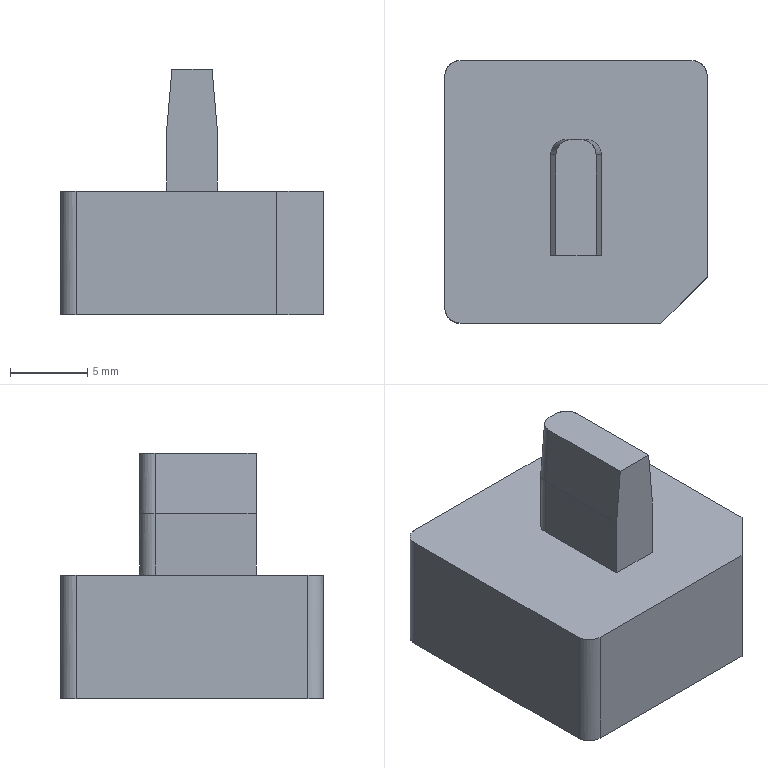NC program | PowerMill | posted with a generic post | part box 17 x 17 x 15.883 mm
Lines 2786 to 3249 of 22972:
N2883 M6
N2884 S8500 M03
N2885 G00 G90 X0.0 Y0.0
N2886 G43 Z11.804 H3
N2887
N2888 G05 P10000 R8
N2889 X11.8334 Y-1.5183
N2890 Z0.8029
N2891 G01 Z-0.3971 F360.0
N2892 X6.5584 F600.0
N2893 X2.4866 Y-1.3941
N2894 X2.4829 Y-1.1993
N2895 X2.4601 Y-1.0057
N2896 X2.0806 Y1.2544
N2897 G03 X-1.4275 Y1.6248 I-1.8056 J-0.3032
N2898 G01 X-2.3187 Y-0.6277
N2899 G03 X-0.431 Y-3.3368 I1.842 J-0.7288
N2900 G01 X0.5523 Y-3.3141
N2901 G03 X2.4866 Y-1.3941 I-0.0457 J1.9804
N2902 G01 X6.5584 Y-1.5183
N2903 G00 Z11.804
N2904 G05 P0
N2905 (---------------)
N2906 ( END TOOLPATH : 粗公基准台01-平坦面偏置-D10 )
N2907 (---------------)
N2908 ( START TOOLPATH : 粗公基准台01-基准面偏置-D10 )
N2909 (---------------)
N2910 G00 X0.0 Y0.0 Z9.8056
N2911 G05 P10000 R8
N2912 X-15.001 Y16.2619
N2913 Z-6.88
N2914 G01 Z-8.08 F360.0
N2915 X-11.5862 Y12.2414 F600.0
N2916 X-6.8885 Y2.4254
N2917 X-6.8737 Y2.7888
N2918 X-6.842 Y3.1512
N2919 G02 X-6.6309 Y4.1515 I5.9397 J-0.7309
N2920 G02 X-6.3033 Y5.0267 I5.8927 J-1.7068
N2921 G01 X-6.1678 Y5.3005
N2922 X-5.9818 Y5.6235
N2923 X-5.7814 Y5.9378
N2924 X-5.6173 Y6.1643
N2925 G02 X-4.8971 Y6.9601 I5.4256 J-4.1864
N2926 G01 X-4.5867 Y7.2255
N2927 X-4.2643 Y7.4761
N2928 X-4.0176 Y7.6439
N2929 G02 X-3.1431 Y8.1122 I3.7067 J-5.8707
N2930 G01 X-2.8431 Y8.234
N2931 G02 X-2.018 Y8.4819 I2.8305 J-7.9259
N2932 G02 X-0.6352 Y8.6371 I1.4581 J-6.7525
N2933 G01 X0.6352
N2934 X1.0035 Y8.6242
N2935 G02 X3.7983 Y7.7732 I-0.3537 J-6.1771
N2936 G02 X4.6028 Y7.212 I-2.6823 J-4.7021
N2937 G02 X6.52 Y4.4929 I-3.9063 J-4.7898
N2938 G02 X6.8891 Y2.3871 I-5.9216 J-2.1229
N2939 G01 Y-4.15
N2940 X6.8744 Y-4.5423
N2941 G02 X6.7574 Y-5.3182 I-6.1404 J0.5287
N2942 G01 X6.6558 Y-5.6975
N2943 X6.5262 Y-6.068
N2944 X6.3691 Y-6.4279
N2945 X6.1857 Y-6.775
N2946 X5.9768 Y-7.1074
N2947 X5.7585 Y-7.4033
N2948 X5.5917 Y-7.6028
N2949 X5.4149 Y-7.7936
N2950 X5.21 Y-7.9985
N2951 X4.9124 Y-8.2546
N2952 X4.5965 Y-8.4877
N2953 G02 X3.917 Y-8.8801 I-3.4465 J5.1847
N2954 G02 X2.8073 Y-9.2684 I-2.3879 J5.0442
N2955 G02 X2.0314 Y-9.3853 I-1.3291 J6.1858
N2956 G01 X1.6391 Y-9.4
N2957 X-1.6391
N2958 G02 X-2.4215 Y-9.3414 I0.0713 J6.2014
N2959 G01 X-2.8073 Y-9.2684
N2960 G02 X-3.5571 Y-9.0371 I1.4757 J6.115
N2961 G02 X-4.2641 Y-8.6966 I2.3236 J5.7292
N2962 G01 X-4.5965 Y-8.4878
N2963 G02 X-5.21 Y-7.9985 I3.6159 J5.1634
N2964 G02 X-5.7437 Y-7.4233 I4.3435 J4.5653
N2965 G01 X-5.9768 Y-7.1074
N2966 X-6.1857 Y-6.775
N2967 X-6.3691 Y-6.4279
N2968 X-6.5261 Y-6.068
N2969 X-6.6558 Y-5.6975
N2970 G02 X-6.8304 Y-4.9325 I6.0732 J1.7886
N2971 G01 X-6.8744 Y-4.5423
N2972 X-6.8891 Y-4.15
N2973 X-6.8885 Y2.4254
N2974 G00 Z9.8056
N2975 G05 P0
N2976 (---------------)
N2977 ( END TOOLPATH : 粗公基准台01-基准面偏置-D10 )
N2978 (---------------)
N2979 ( START TOOLPATH : 粗公基准台01-基准台侧光-D10 )
N2980 (---------------)
N2981 G00 X0.0 Y0.0 Z9.8056
N2982 G05 P10000 R8
N2983 X13.4803 Y-14.7747
N2984 Z-14.78
N2985 G01 Z-15.98 F360.0
N2986 G03 X9.9447 Y-11.2392 I-1.7678 J1.7678 F600.0
N2987 G01 X9.0587 Y-12.1252
N2988 X9.0582 Y-12.1257
N2989 X9.0577 Y-12.1262
N2990 X8.9953 Y-12.1864
N2991 X8.9933 Y-12.1883
N2992 X8.9913 Y-12.19
N2993 X8.5443 Y-12.5666
N2994 X8.5408 Y-12.5694
N2995 X8.5371 Y-12.572
N2996 X8.0901 Y-12.87
N2997 X8.0872 Y-12.8719
N2998 X8.0842 Y-12.8736
N2999 X7.7935 Y-13.0328
N3000 X7.7918 Y-13.0337
N3001 X7.79 Y-13.0346
N3002 X7.6336 Y-13.1102
N3003 X7.6312 Y-13.1114
N3004 X7.6288 Y-13.1124
N3005 X7.1818 Y-13.2935
N3006 X7.1783 Y-13.2948
N3007 X7.1746 Y-13.296
N3008 X6.7277 Y-13.4293
N3009 X6.7248 Y-13.4301
N3010 X6.722 Y-13.4308
N3011 X6.4639 Y-13.4877
N3012 X6.4621 Y-13.4881
N3013 X6.4603 Y-13.4884
N3014 X6.2714 Y-13.5211
N3015 X6.2689 Y-13.5215
N3016 X6.2664 Y-13.5218
N3017 X5.8194 Y-13.5699
N3018 X5.816 Y-13.5702
N3019 X5.8125 Y-13.5704
N3020 X5.3656 Y-13.58
N3021 X5.3647
N3022 X5.3638
N3023 X-7.5988 Y-13.5791
N3024 X-7.6011 Y-13.579
N3025 X-7.6033 Y-13.5789
N3026 X-8.0503 Y-13.5532
N3027 X-8.053 Y-13.553
N3028 X-8.0557 Y-13.5527
N3029 X-8.5027 Y-13.4965
N3030 X-8.5059 Y-13.496
N3031 X-8.5091 Y-13.4954
N3032 X-8.9561 Y-13.4017
N3033 X-8.9589 Y-13.4011
N3034 X-8.9617 Y-13.4003
N3035 X-9.4087 Y-13.2723
N3036 X-9.4118 Y-13.2713
N3037 X-9.4148 Y-13.2703
N3038 X-9.8618 Y-13.1025
N3039 X-9.8649 Y-13.1013
N3040 X-9.8679 Y-13.0999
N3041 X-10.3149 Y-12.8887
N3042 X-10.3178 Y-12.8872
N3043 X-10.3208 Y-12.8856
N3044 X-10.7677 Y-12.6268
N3045 X-10.7708 Y-12.6249
N3046 X-10.7738 Y-12.6229
N3047 X-11.2208 Y-12.3073
N3048 X-11.2238 Y-12.3051
N3049 X-11.2266 Y-12.3027
N3050 X-11.6736 Y-11.9205
N3051 X-11.676 Y-11.9184
N3052 X-11.6782 Y-11.9163
N3053 X-11.9163 Y-11.6782
N3054 X-11.9184 Y-11.676
N3055 X-11.9205 Y-11.6736
N3056 X-12.3027 Y-11.2266
N3057 X-12.3049 Y-11.224
N3058 X-12.307 Y-11.2213
N3059 X-12.5806 Y-10.8396
N3060 X-12.5827 Y-10.8365
N3061 X-12.5846 Y-10.8334
N3062 X-12.8853 Y-10.3212
N3063 X-12.8871 Y-10.318
N3064 X-12.8887 Y-10.3149
N3065 X-13.0999 Y-9.8679
N3066 X-13.1013 Y-9.8649
N3067 X-13.1025 Y-9.8618
N3068 X-13.2703 Y-9.4148
N3069 X-13.2713 Y-9.4118
N3070 X-13.2723 Y-9.4087
N3071 X-13.4003 Y-8.9617
N3072 X-13.4011 Y-8.9591
N3073 X-13.4017 Y-8.9564
N3074 X-13.4878 Y-8.5527
N3075 X-13.4884 Y-8.5495
N3076 X-13.4889 Y-8.5463
N3077 X-13.5527 Y-8.0561
N3078 X-13.553 Y-8.0532
N3079 X-13.5532 Y-8.0503
N3080 X-13.5789 Y-7.6033
N3081 X-13.579 Y-7.6011
N3082 X-13.5791 Y-7.5988
N3083 Y0.0
N3084 Y7.5988
N3085 X-13.579 Y7.6011
N3086 X-13.5789 Y7.6033
N3087 X-13.5532 Y8.0503
N3088 X-13.553 Y8.053
N3089 X-13.5527 Y8.0557
N3090 X-13.4965 Y8.5027
N3091 X-13.496 Y8.5059
N3092 X-13.4954 Y8.5091
N3093 X-13.4017 Y8.9561
N3094 X-13.4011 Y8.9589
N3095 X-13.4003 Y8.9617
N3096 X-13.2723 Y9.4087
N3097 X-13.2713 Y9.4118
N3098 X-13.2703 Y9.4148
N3099 X-13.1025 Y9.8618
N3100 X-13.1013 Y9.8649
N3101 X-13.0999 Y9.8679
N3102 X-12.8887 Y10.3149
N3103 X-12.8872 Y10.3178
N3104 X-12.8856 Y10.3208
N3105 X-12.6268 Y10.7677
N3106 X-12.6249 Y10.7708
N3107 X-12.6229 Y10.7738
N3108 X-12.3073 Y11.2208
N3109 X-12.3051 Y11.2238
N3110 X-12.3027 Y11.2266
N3111 X-11.9205 Y11.6736
N3112 X-11.9184 Y11.676
N3113 X-11.9163 Y11.6782
N3114 X-11.6782 Y11.9163
N3115 X-11.676 Y11.9184
N3116 X-11.6736 Y11.9205
N3117 X-11.2266 Y12.3027
N3118 X-11.224 Y12.3049
N3119 X-11.2213 Y12.307
N3120 X-10.8396 Y12.5806
N3121 X-10.8365 Y12.5827
N3122 X-10.8334 Y12.5846
N3123 X-10.3212 Y12.8853
N3124 X-10.318 Y12.8871
N3125 X-10.3149 Y12.8887
N3126 X-9.8679 Y13.0999
N3127 X-9.8649 Y13.1013
N3128 X-9.8618 Y13.1025
N3129 X-9.4148 Y13.2703
N3130 X-9.4118 Y13.2713
N3131 X-9.4087 Y13.2723
N3132 X-8.9617 Y13.4003
N3133 X-8.9591 Y13.4011
N3134 X-8.9564 Y13.4017
N3135 X-8.5527 Y13.4878
N3136 X-8.5495 Y13.4884
N3137 X-8.5463 Y13.4889
N3138 X-8.0561 Y13.5527
N3139 X-8.0532 Y13.553
N3140 X-8.0503 Y13.5532
N3141 X-7.6033 Y13.5789
N3142 X-7.6011 Y13.579
N3143 X-7.5988 Y13.5791
N3144 X7.5988
N3145 X7.6011 Y13.579
N3146 X7.6033 Y13.5789
N3147 X8.0503 Y13.5532
N3148 X8.053 Y13.553
N3149 X8.0557 Y13.5527
N3150 X8.5027 Y13.4965
N3151 X8.5059 Y13.496
N3152 X8.5091 Y13.4954
N3153 X8.9561 Y13.4017
N3154 X8.9589 Y13.4011
N3155 X8.9617 Y13.4003
N3156 X9.4087 Y13.2723
N3157 X9.4118 Y13.2713
N3158 X9.4148 Y13.2703
N3159 X9.8618 Y13.1025
N3160 X9.8649 Y13.1013
N3161 X9.8679 Y13.0999
N3162 X10.3149 Y12.8887
N3163 X10.3178 Y12.8872
N3164 X10.3208 Y12.8856
N3165 X10.7677 Y12.6268
N3166 X10.7708 Y12.6249
N3167 X10.7738 Y12.6229
N3168 X11.2208 Y12.3073
N3169 X11.2238 Y12.3051
N3170 X11.2266 Y12.3027
N3171 X11.6736 Y11.9205
N3172 X11.676 Y11.9184
N3173 X11.6782 Y11.9163
N3174 X11.9163 Y11.6782
N3175 X11.9184 Y11.676
N3176 X11.9205 Y11.6736
N3177 X12.3027 Y11.2266
N3178 X12.3049 Y11.224
N3179 X12.307 Y11.2213
N3180 X12.5806 Y10.8396
N3181 X12.5827 Y10.8365
N3182 X12.5846 Y10.8334
N3183 X12.8853 Y10.3212
N3184 X12.8871 Y10.318
N3185 X12.8887 Y10.3149
N3186 X13.0999 Y9.8679
N3187 X13.1013 Y9.8649
N3188 X13.1025 Y9.8618
N3189 X13.2703 Y9.4148
N3190 X13.2713 Y9.4118
N3191 X13.2723 Y9.4087
N3192 X13.4003 Y8.9617
N3193 X13.4011 Y8.9591
N3194 X13.4017 Y8.9564
N3195 X13.4878 Y8.5527
N3196 X13.4884 Y8.5495
N3197 X13.4889 Y8.5463
N3198 X13.5527 Y8.0561
N3199 X13.553 Y8.0532
N3200 X13.5532 Y8.0503
N3201 X13.5789 Y7.6033
N3202 X13.579 Y7.6011
N3203 X13.5791 Y7.5988
N3204 X13.58 Y-5.3638
N3205 Y-5.3647
N3206 Y-5.3656
N3207 X13.5703 Y-5.8125
N3208 X13.5702 Y-5.816
N3209 X13.5699 Y-5.8194
N3210 X13.5218 Y-6.2664
N3211 X13.5215 Y-6.2689
N3212 X13.5211 Y-6.2714
N3213 X13.4884 Y-6.4603
N3214 X13.4881 Y-6.4621
N3215 X13.4877 Y-6.4639
N3216 X13.4308 Y-6.722
N3217 X13.4301 Y-6.7248
N3218 X13.4294 Y-6.7277
N3219 X13.296 Y-7.1746
N3220 X13.2948 Y-7.1783
N3221 X13.2935 Y-7.1818
N3222 X13.1124 Y-7.6288
N3223 X13.1113 Y-7.6312
N3224 X13.1102 Y-7.6336
N3225 X13.0346 Y-7.7899
N3226 X13.0337 Y-7.7918
N3227 X13.0328 Y-7.7935
N3228 X12.8736 Y-8.0842
N3229 X12.8719 Y-8.0871
N3230 X12.8701 Y-8.09
N3231 X12.5822 Y-8.5234
N3232 X12.5797 Y-8.527
N3233 X12.5769 Y-8.5305
N3234 X12.1901 Y-8.9912
N3235 X12.1883 Y-8.9932
N3236 X12.1864 Y-8.9952
N3237 X12.1262 Y-9.0577
N3238 X12.1257 Y-9.0582
N3239 X12.1252 Y-9.0587
N3240 X9.9447 Y-11.2392
N3241 G03 X13.4803 Y-14.7747 I1.7678 J-1.7677
N3242 G01 X13.4288 Y-14.713
N3243 G03 X9.8933 Y-11.1775 I-1.7678 J1.7677
N3244 G01 X9.0022 Y-12.0686
N3245 X8.9397 Y-12.1289
N3246 X8.4927 Y-12.5055
N3247 X8.0457 Y-12.8034
N3248 X7.7551 Y-12.9626
N3249 X7.5988 Y-13.0382
N3250 X7.1518 Y-13.2193
N3251 X6.7048 Y-13.3527
N3252 X6.4467 Y-13.4096
N3253 X6.2578 Y-13.4422
N3254 X5.8108 Y-13.4904
N3255 X5.3638 Y-13.5
N3256 X-7.5988 Y-13.4991
N3257 X-8.0457 Y-13.4734
N3258 X-8.4927 Y-13.4171
N3259 X-8.9397 Y-13.3234
N3260 X-9.3867 Y-13.1954
N3261 X-9.8337 Y-13.0276
N3262 X-10.2807 Y-12.8163
N3263 X-10.7277 Y-12.5576
N3264 X-11.1746 Y-12.2419
N3265 X-11.6216 Y-11.8597
N3266 X-11.8597 Y-11.6216
N3267 X-12.2419 Y-11.1746
N3268 X-12.5156 Y-10.7929
N3269 X-12.8163 Y-10.2807
N3270 X-13.0276 Y-9.8337
N3271 X-13.1954 Y-9.3867
N3272 X-13.3234 Y-8.9397
N3273 X-13.4096 Y-8.536
N3274 X-13.4734 Y-8.0457
N3275 X-13.4991 Y-7.5988
N3276 Y0.0
N3277 Y7.5988
N3278 X-13.4734 Y8.0457
N3279 X-13.4171 Y8.4927
N3280 X-13.3234 Y8.9397
N3281 X-13.1954 Y9.3867
N3282 X-13.0276 Y9.8337
N3283 X-12.8163 Y10.2807
N3284 X-12.5576 Y10.7277
N3285 X-12.2419 Y11.1746
N3286 X-11.8597 Y11.6216
N3287 X-11.6216 Y11.8597
N3288 X-11.1746 Y12.2419
N3289 X-10.7929 Y12.5156
N3290 X-10.2807 Y12.8163
N3291 X-9.8337 Y13.0276
N3292 X-9.3867 Y13.1954
N3293 X-8.9397 Y13.3234
N3294 X-8.536 Y13.4096
N3295 X-8.0457 Y13.4734
N3296 X-7.5988 Y13.4991
N3297 X7.5988
N3298 X8.0457 Y13.4734
N3299 X8.4927 Y13.4171
N3300 X8.9397 Y13.3234
N3301 X9.3867 Y13.1954
N3302 X9.8337 Y13.0276
N3303 X10.2807 Y12.8163
N3304 X10.7277 Y12.5576
N3305 X11.1746 Y12.2419
N3306 X11.6216 Y11.8597
N3307 X11.8597 Y11.6216
N3308 X12.2419 Y11.1746
N3309 X12.5156 Y10.7929
N3310 X12.8163 Y10.2807
N3311 X13.0276 Y9.8337
N3312 X13.1954 Y9.3867
N3313 X13.3234 Y8.9397
N3314 X13.4096 Y8.536
N3315 X13.4734 Y8.0457
N3316 X13.4991 Y7.5988
N3317 X13.5 Y-5.3638
N3318 X13.4904 Y-5.8108
N3319 X13.4423 Y-6.2578
N3320 X13.4096 Y-6.4467
N3321 X13.3527 Y-6.7048
N3322 X13.2193 Y-7.1518
N3323 X13.0382 Y-7.5988
N3324 X12.9626 Y-7.7551
N3325 X12.8034 Y-8.0457
N3326 X12.5156 Y-8.4791
N3327 X12.1288 Y-8.9397
N3328 X12.0686 Y-9.0022
N3329 X9.8933 Y-11.1775
N3330 G03 X13.4288 Y-14.713 I1.7677 J-1.7678
N3331 G00 Z9.8056
N3332 G05 P0
N3333 (---------------)
N3334 ( END TOOLPATH : 粗公基准台01-基准台侧光-D10 )
N3335 (---------------)
N3336
N3337 M05
N3338 G53 Z0.0
N3339 (---------------)
N3340 ( START TOOLPATH : 粗公精光01-等高-D4 )
N3341 (---------------)
N3342 ( TOOL NO.    :14 )
N3343 ( TOOL TYPE   : ENDMILL)
N3344 ( TOOL ID     : D4_2_1)
N3345 ( TOOL DIA    : 4.0 LENGTH 62.92)
N3346 T14